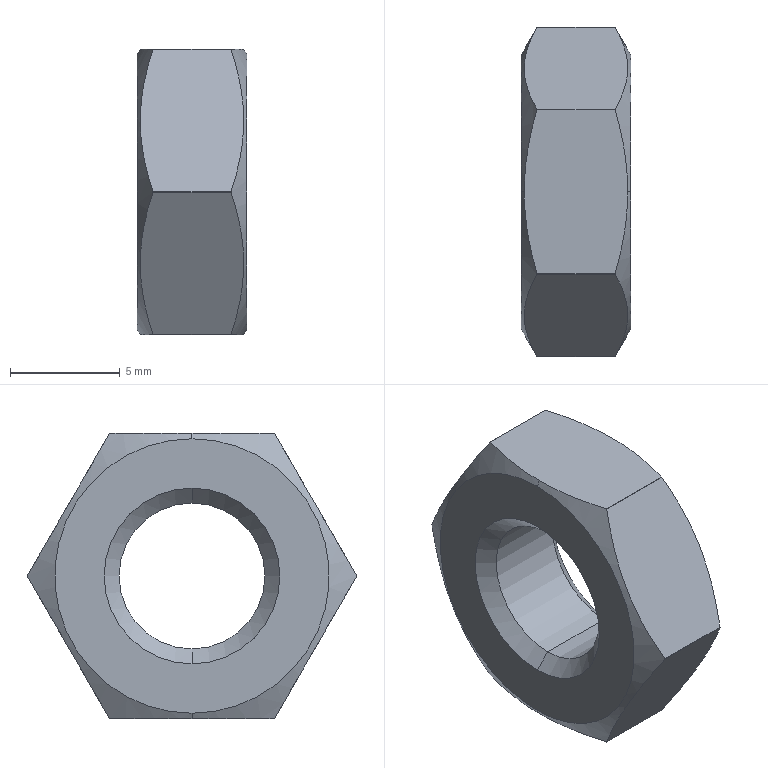Part | STEP file | Guide wheel mechanism revised.sldasm-Part-424 | 1 solid | 24 faces | box 5 x 15 x 13 mm | volume 537.919 mm3 | cone 8 | cylinder 8 | plane 8 | commonest cylinder face diameters 15 x6 6.647 x2
STEP:
#1=CARTESIAN_POINT('',(4.324,0.,-3.324));
#2=VERTEX_POINT('',#1);
#3=CARTESIAN_POINT('',(4.324,0.,3.324));
#4=VERTEX_POINT('',#3);
#5=CARTESIAN_POINT('',(4.324,0.,0.));
#6=DIRECTION('',(-1.,0.,0.));
#7=DIRECTION('',(0.,0.,1.));
#8=AXIS2_PLACEMENT_3D('',#5,#6,#7);
#9=CIRCLE('',#8,3.324);
#10=EDGE_CURVE('',#2,#4,#9,.T.);
#11=ORIENTED_EDGE('',*,*,#10,.T.);
#12=CARTESIAN_POINT('',(5.,0.,4.));
#13=VERTEX_POINT('',#12);
#14=CARTESIAN_POINT('',(5.,0.,4.));
#15=DIRECTION('',(0.7071,0.,0.7071));
#16=VECTOR('',#15,1000.);
#17=LINE('',#14,#16);
#18=EDGE_CURVE('',#4,#13,#17,.T.);
#19=ORIENTED_EDGE('',*,*,#18,.T.);
#20=CARTESIAN_POINT('',(5.,0.,-4.));
#21=VERTEX_POINT('',#20);
#22=CARTESIAN_POINT('',(5.,0.,0.));
#23=DIRECTION('',(-1.,0.,0.));
#24=DIRECTION('',(0.,0.,1.));
#25=AXIS2_PLACEMENT_3D('',#22,#23,#24);
#26=CIRCLE('',#25,4.);
#27=EDGE_CURVE('',#21,#13,#26,.T.);
#28=ORIENTED_EDGE('',*,*,#27,.F.);
#29=CARTESIAN_POINT('',(5.,0.,-4.));
#30=DIRECTION('',(0.7071,0.,-0.7071));
#31=VECTOR('',#30,1000.);
#32=LINE('',#29,#31);
#33=EDGE_CURVE('',#2,#21,#32,.T.);
#34=ORIENTED_EDGE('',*,*,#33,.F.);
#35=EDGE_LOOP('',(#11,#19,#28,#34));
#36=FACE_OUTER_BOUND('',#35,.T.);
#37=CARTESIAN_POINT('',(5.,0.,0.));
#38=DIRECTION('',(1.,0.,0.));
#39=DIRECTION('',(0.,0.,-1.));
#40=AXIS2_PLACEMENT_3D('',#37,#38,#39);
#41=CONICAL_SURFACE('',#40,4.,0.7854);
#42=ADVANCED_FACE('',(#36),#41,.F.);
#43=ORIENTED_EDGE('',*,*,#10,.F.);
#44=CARTESIAN_POINT('',(0.6765,0.,-3.324));
#45=VERTEX_POINT('',#44);
#46=CARTESIAN_POINT('',(5.,0.,-3.324));
#47=DIRECTION('',(-1.,0.,0.));
#48=VECTOR('',#47,1000.);
#49=LINE('',#46,#48);
#50=EDGE_CURVE('',#2,#45,#49,.T.);
#51=ORIENTED_EDGE('',*,*,#50,.T.);
#52=CARTESIAN_POINT('',(0.6765,0.,3.324));
#53=VERTEX_POINT('',#52);
#54=CARTESIAN_POINT('',(0.6765,0.,0.));
#55=DIRECTION('',(-1.,0.,0.));
#56=DIRECTION('',(0.,0.,1.));
#57=AXIS2_PLACEMENT_3D('',#54,#55,#56);
#58=CIRCLE('',#57,3.324);
#59=EDGE_CURVE('',#45,#53,#58,.T.);
#60=ORIENTED_EDGE('',*,*,#59,.T.);
#61=CARTESIAN_POINT('',(5.,0.,3.324));
#62=DIRECTION('',(-1.,0.,0.));
#63=VECTOR('',#62,1000.);
#64=LINE('',#61,#63);
#65=EDGE_CURVE('',#4,#53,#64,.T.);
#66=ORIENTED_EDGE('',*,*,#65,.F.);
#67=EDGE_LOOP('',(#43,#51,#60,#66));
#68=FACE_OUTER_BOUND('',#67,.T.);
#69=CARTESIAN_POINT('',(5.,0.,0.));
#70=DIRECTION('',(-1.,0.,0.));
#71=DIRECTION('',(0.,0.,1.));
#72=AXIS2_PLACEMENT_3D('',#69,#70,#71);
#73=CYLINDRICAL_SURFACE('',#72,3.324);
#74=ADVANCED_FACE('',(#68),#73,.F.);
#75=ORIENTED_EDGE('',*,*,#59,.F.);
#76=CARTESIAN_POINT('',(0.,0.,-4.));
#77=VERTEX_POINT('',#76);
#78=CARTESIAN_POINT('',(0.6765,0.,-3.324));
#79=DIRECTION('',(-0.7071,0.,-0.7071));
#80=VECTOR('',#79,1000.);
#81=LINE('',#78,#80);
#82=EDGE_CURVE('',#45,#77,#81,.T.);
#83=ORIENTED_EDGE('',*,*,#82,.T.);
#84=CARTESIAN_POINT('',(0.,0.,4.));
#85=VERTEX_POINT('',#84);
#86=CARTESIAN_POINT('',(0.,0.,0.));
#87=DIRECTION('',(-1.,0.,0.));
#88=DIRECTION('',(0.,0.,1.));
#89=AXIS2_PLACEMENT_3D('',#86,#87,#88);
#90=CIRCLE('',#89,4.);
#91=EDGE_CURVE('',#77,#85,#90,.T.);
#92=ORIENTED_EDGE('',*,*,#91,.T.);
#93=CARTESIAN_POINT('',(0.6765,0.,3.324));
#94=DIRECTION('',(-0.7071,0.,0.7071));
#95=VECTOR('',#94,1000.);
#96=LINE('',#93,#95);
#97=EDGE_CURVE('',#53,#85,#96,.T.);
#98=ORIENTED_EDGE('',*,*,#97,.F.);
#99=EDGE_LOOP('',(#75,#83,#92,#98));
#100=FACE_OUTER_BOUND('',#99,.T.);
#101=CARTESIAN_POINT('',(0.6765,0.,0.));
#102=DIRECTION('',(-1.,0.,0.));
#103=DIRECTION('',(0.,0.,1.));
#104=AXIS2_PLACEMENT_3D('',#101,#102,#103);
#105=CONICAL_SURFACE('',#104,3.324,0.7854);
#106=ADVANCED_FACE('',(#100),#105,.F.);
#107=CARTESIAN_POINT('',(5.,0.,6.25));
#108=VERTEX_POINT('',#107);
#109=CARTESIAN_POINT('',(5.,0.,-6.25));
#110=VERTEX_POINT('',#109);
#111=CARTESIAN_POINT('',(5.,0.,0.));
#112=DIRECTION('',(-1.,0.,0.));
#113=DIRECTION('',(0.,0.,1.));
#114=AXIS2_PLACEMENT_3D('',#111,#112,#113);
#115=CIRCLE('',#114,6.25);
#116=EDGE_CURVE('',#108,#110,#115,.T.);
#117=ORIENTED_EDGE('',*,*,#116,.T.);
#118=CARTESIAN_POINT('',(4.856,0.,-6.5));
#119=VERTEX_POINT('',#118);
#120=CARTESIAN_POINT('',(5.,0.,-6.25));
#121=DIRECTION('',(-0.5,0.,-0.866));
#122=VECTOR('',#121,1000.);
#123=LINE('',#120,#122);
#124=EDGE_CURVE('',#110,#119,#123,.T.);
#125=ORIENTED_EDGE('',*,*,#124,.T.);
#126=CARTESIAN_POINT('',(4.278,3.742,-6.5));
#127=VERTEX_POINT('',#126);
#128=CARTESIAN_POINT('',(4.856,0.,-6.5));
#129=CARTESIAN_POINT('',(4.856,0.6325,-6.5));
#130=CARTESIAN_POINT('',(4.8,1.274,-6.5));
#131=CARTESIAN_POINT('',(4.598,2.524,-6.5));
#132=CARTESIAN_POINT('',(4.453,3.137,-6.5));
#133=CARTESIAN_POINT('',(4.278,3.742,-6.5));
#134=B_SPLINE_CURVE_WITH_KNOTS('',3,(#128,#129,#130,#131,#132,#133),.UNSPECIFIED.,.F.,.F.,(4,2,4),(0.01047,0.01236,0.01426),.UNSPECIFIED.);
#135=EDGE_CURVE('',#119,#127,#134,.T.);
#136=ORIENTED_EDGE('',*,*,#135,.T.);
#137=CARTESIAN_POINT('',(4.278,3.758,-6.49));
#138=VERTEX_POINT('',#137);
#139=CARTESIAN_POINT('',(4.278,0.,0.));
#140=DIRECTION('',(-1.,0.,0.));
#141=DIRECTION('',(0.,0.,1.));
#142=AXIS2_PLACEMENT_3D('',#139,#140,#141);
#143=CIRCLE('',#142,7.5);
#144=EDGE_CURVE('',#138,#127,#143,.T.);
#145=ORIENTED_EDGE('',*,*,#144,.F.);
#146=CARTESIAN_POINT('',(4.278,7.5,-0.00963));
#147=VERTEX_POINT('',#146);
#148=CARTESIAN_POINT('',(4.278,3.758,-6.49));
#149=CARTESIAN_POINT('',(4.454,4.064,-5.961));
#150=CARTESIAN_POINT('',(4.599,4.372,-5.428));
#151=CARTESIAN_POINT('',(4.8,4.993,-4.351));
#152=CARTESIAN_POINT('',(4.855,5.307,-3.807));
#153=CARTESIAN_POINT('',(4.856,5.785,-2.981));
#154=CARTESIAN_POINT('',(4.842,5.944,-2.704));
#155=CARTESIAN_POINT('',(4.79,6.26,-2.157));
#156=CARTESIAN_POINT('',(4.751,6.417,-1.885));
#157=CARTESIAN_POINT('',(4.6,6.886,-1.074));
#158=CARTESIAN_POINT('',(4.455,7.194,-0.5394));
#159=CARTESIAN_POINT('',(4.278,7.5,-0.00963));
#160=B_SPLINE_CURVE_WITH_KNOTS('',3,(#148,#149,#150,#151,#152,#153,#154,#155,#156,#157,#158,#159),.UNSPECIFIED.,.F.,.F.,(4,2,2,2,2,4),(0.000000716,0.00189,0.003779,0.004724,0.005668,0.007558),.UNSPECIFIED.);
#161=EDGE_CURVE('',#138,#147,#160,.T.);
#162=ORIENTED_EDGE('',*,*,#161,.T.);
#163=CARTESIAN_POINT('',(4.278,7.5,0.00963));
#164=VERTEX_POINT('',#163);
#165=CARTESIAN_POINT('',(4.278,0.,0.));
#166=DIRECTION('',(-1.,0.,0.));
#167=DIRECTION('',(0.,0.,1.));
#168=AXIS2_PLACEMENT_3D('',#165,#166,#167);
#169=CIRCLE('',#168,7.5);
#170=EDGE_CURVE('',#164,#147,#169,.T.);
#171=ORIENTED_EDGE('',*,*,#170,.F.);
#172=CARTESIAN_POINT('',(4.278,3.758,6.49));
#173=VERTEX_POINT('',#172);
#174=CARTESIAN_POINT('',(4.278,7.5,0.00963));
#175=CARTESIAN_POINT('',(4.454,7.194,0.5388));
#176=CARTESIAN_POINT('',(4.599,6.887,1.072));
#177=CARTESIAN_POINT('',(4.8,6.265,2.149));
#178=CARTESIAN_POINT('',(4.855,5.951,2.693));
#179=CARTESIAN_POINT('',(4.856,5.474,3.519));
#180=CARTESIAN_POINT('',(4.842,5.314,3.796));
#181=CARTESIAN_POINT('',(4.79,4.998,4.343));
#182=CARTESIAN_POINT('',(4.751,4.841,4.615));
#183=CARTESIAN_POINT('',(4.6,4.373,5.426));
#184=CARTESIAN_POINT('',(4.455,4.064,5.961));
#185=CARTESIAN_POINT('',(4.278,3.758,6.49));
#186=B_SPLINE_CURVE_WITH_KNOTS('',3,(#174,#175,#176,#177,#178,#179,#180,#181,#182,#183,#184,#185),.UNSPECIFIED.,.F.,.F.,(4,2,2,2,2,4),(0.000000425,0.00189,0.003779,0.004723,0.005668,0.007557),.UNSPECIFIED.);
#187=EDGE_CURVE('',#164,#173,#186,.T.);
#188=ORIENTED_EDGE('',*,*,#187,.T.);
#189=CARTESIAN_POINT('',(4.278,3.742,6.5));
#190=VERTEX_POINT('',#189);
#191=CARTESIAN_POINT('',(4.278,0.,0.));
#192=DIRECTION('',(-1.,0.,0.));
#193=DIRECTION('',(0.,0.,1.));
#194=AXIS2_PLACEMENT_3D('',#191,#192,#193);
#195=CIRCLE('',#194,7.5);
#196=EDGE_CURVE('',#190,#173,#195,.T.);
#197=ORIENTED_EDGE('',*,*,#196,.F.);
#198=CARTESIAN_POINT('',(4.856,0.,6.5));
#199=VERTEX_POINT('',#198);
#200=CARTESIAN_POINT('',(4.278,3.742,6.5));
#201=CARTESIAN_POINT('',(4.453,3.137,6.5));
#202=CARTESIAN_POINT('',(4.598,2.524,6.5));
#203=CARTESIAN_POINT('',(4.8,1.274,6.5));
#204=CARTESIAN_POINT('',(4.856,0.6325,6.5));
#205=CARTESIAN_POINT('',(4.856,0.,6.5));
#206=B_SPLINE_CURVE_WITH_KNOTS('',3,(#200,#201,#202,#203,#204,#205),.UNSPECIFIED.,.F.,.F.,(4,2,4),(0.002787,0.004676,0.006564),.UNSPECIFIED.);
#207=EDGE_CURVE('',#190,#199,#206,.T.);
#208=ORIENTED_EDGE('',*,*,#207,.T.);
#209=CARTESIAN_POINT('',(5.,0.,6.25));
#210=DIRECTION('',(-0.5,0.,0.866));
#211=VECTOR('',#210,1000.);
#212=LINE('',#209,#211);
#213=EDGE_CURVE('',#108,#199,#212,.T.);
#214=ORIENTED_EDGE('',*,*,#213,.F.);
#215=EDGE_LOOP('',(#117,#125,#136,#145,#162,#171,#188,#197,#208,#214));
#216=FACE_OUTER_BOUND('',#215,.T.);
#217=CARTESIAN_POINT('',(5.,0.,0.));
#218=DIRECTION('',(-1.,0.,0.));
#219=DIRECTION('',(0.,0.,1.));
#220=AXIS2_PLACEMENT_3D('',#217,#218,#219);
#221=CONICAL_SURFACE('',#220,6.25,1.047);
#222=ADVANCED_FACE('',(#216),#221,.T.);
#223=CARTESIAN_POINT('',(0.,0.,6.25));
#224=VERTEX_POINT('',#223);
#225=CARTESIAN_POINT('',(0.,0.,-6.25));
#226=VERTEX_POINT('',#225);
#227=CARTESIAN_POINT('',(0.,0.,0.));
#228=DIRECTION('',(-1.,0.,0.));
#229=DIRECTION('',(0.,0.,1.));
#230=AXIS2_PLACEMENT_3D('',#227,#228,#229);
#231=CIRCLE('',#230,6.25);
#232=EDGE_CURVE('',#224,#226,#231,.T.);
#233=ORIENTED_EDGE('',*,*,#232,.F.);
#234=CARTESIAN_POINT('',(0.1443,0.,6.5));
#235=VERTEX_POINT('',#234);
#236=CARTESIAN_POINT('',(0.7217,0.,7.5));
#237=DIRECTION('',(0.5,0.,0.866));
#238=VECTOR('',#237,1000.);
#239=LINE('',#236,#238);
#240=EDGE_CURVE('',#224,#235,#239,.T.);
#241=ORIENTED_EDGE('',*,*,#240,.T.);
#242=CARTESIAN_POINT('',(0.7217,3.742,6.5));
#243=VERTEX_POINT('',#242);
#244=CARTESIAN_POINT('',(0.1443,0.,6.5));
#245=CARTESIAN_POINT('',(0.1443,0.6325,6.5));
#246=CARTESIAN_POINT('',(0.2,1.274,6.5));
#247=CARTESIAN_POINT('',(0.4023,2.524,6.5));
#248=CARTESIAN_POINT('',(0.5474,3.137,6.5));
#249=CARTESIAN_POINT('',(0.7217,3.742,6.5));
#250=B_SPLINE_CURVE_WITH_KNOTS('',3,(#244,#245,#246,#247,#248,#249),.UNSPECIFIED.,.F.,.F.,(4,2,4),(0.01047,0.01236,0.01426),.UNSPECIFIED.);
#251=EDGE_CURVE('',#235,#243,#250,.T.);
#252=ORIENTED_EDGE('',*,*,#251,.T.);
#253=CARTESIAN_POINT('',(0.7217,3.758,6.49));
#254=VERTEX_POINT('',#253);
#255=CARTESIAN_POINT('',(0.7217,0.,0.));
#256=DIRECTION('',(-1.,0.,0.));
#257=DIRECTION('',(0.,0.,1.));
#258=AXIS2_PLACEMENT_3D('',#255,#256,#257);
#259=CIRCLE('',#258,7.5);
#260=EDGE_CURVE('',#243,#254,#259,.T.);
#261=ORIENTED_EDGE('',*,*,#260,.T.);
#262=CARTESIAN_POINT('',(0.7217,7.5,0.00963));
#263=VERTEX_POINT('',#262);
#264=CARTESIAN_POINT('',(0.7217,3.758,6.49));
#265=CARTESIAN_POINT('',(0.5457,4.064,5.961));
#266=CARTESIAN_POINT('',(0.4007,4.372,5.428));
#267=CARTESIAN_POINT('',(0.1999,4.993,4.351));
#268=CARTESIAN_POINT('',(0.1448,5.307,3.807));
#269=CARTESIAN_POINT('',(0.1441,5.785,2.981));
#270=CARTESIAN_POINT('',(0.1576,5.944,2.704));
#271=CARTESIAN_POINT('',(0.2102,6.26,2.157));
#272=CARTESIAN_POINT('',(0.2493,6.417,1.885));
#273=CARTESIAN_POINT('',(0.4001,6.886,1.074));
#274=CARTESIAN_POINT('',(0.5455,7.194,0.5394));
#275=CARTESIAN_POINT('',(0.7217,7.5,0.00963));
#276=B_SPLINE_CURVE_WITH_KNOTS('',3,(#264,#265,#266,#267,#268,#269,#270,#271,#272,#273,#274,#275),.UNSPECIFIED.,.F.,.F.,(4,2,2,2,2,4),(0.000000716,0.00189,0.003779,0.004724,0.005668,0.007558),.UNSPECIFIED.);
#277=EDGE_CURVE('',#254,#263,#276,.T.);
#278=ORIENTED_EDGE('',*,*,#277,.T.);
#279=CARTESIAN_POINT('',(0.7217,7.5,-0.00963));
#280=VERTEX_POINT('',#279);
#281=CARTESIAN_POINT('',(0.7217,0.,0.));
#282=DIRECTION('',(-1.,0.,0.));
#283=DIRECTION('',(0.,0.,1.));
#284=AXIS2_PLACEMENT_3D('',#281,#282,#283);
#285=CIRCLE('',#284,7.5);
#286=EDGE_CURVE('',#263,#280,#285,.T.);
#287=ORIENTED_EDGE('',*,*,#286,.T.);
#288=CARTESIAN_POINT('',(0.7217,3.758,-6.49));
#289=VERTEX_POINT('',#288);
#290=CARTESIAN_POINT('',(0.7217,7.5,-0.00963));
#291=CARTESIAN_POINT('',(0.5457,7.194,-0.5388));
#292=CARTESIAN_POINT('',(0.4007,6.887,-1.072));
#293=CARTESIAN_POINT('',(0.1999,6.265,-2.149));
#294=CARTESIAN_POINT('',(0.1448,5.951,-2.693));
#295=CARTESIAN_POINT('',(0.1441,5.474,-3.519));
#296=CARTESIAN_POINT('',(0.1576,5.314,-3.796));
#297=CARTESIAN_POINT('',(0.2102,4.998,-4.343));
#298=CARTESIAN_POINT('',(0.2493,4.841,-4.615));
#299=CARTESIAN_POINT('',(0.4001,4.373,-5.426));
#300=CARTESIAN_POINT('',(0.5455,4.064,-5.961));
#301=CARTESIAN_POINT('',(0.7217,3.758,-6.49));
#302=B_SPLINE_CURVE_WITH_KNOTS('',3,(#290,#291,#292,#293,#294,#295,#296,#297,#298,#299,#300,#301),.UNSPECIFIED.,.F.,.F.,(4,2,2,2,2,4),(0.000000425,0.00189,0.003779,0.004723,0.005668,0.007557),.UNSPECIFIED.);
#303=EDGE_CURVE('',#280,#289,#302,.T.);
#304=ORIENTED_EDGE('',*,*,#303,.T.);
#305=CARTESIAN_POINT('',(0.7217,3.742,-6.5));
#306=VERTEX_POINT('',#305);
#307=CARTESIAN_POINT('',(0.7217,0.,0.));
#308=DIRECTION('',(-1.,0.,0.));
#309=DIRECTION('',(0.,0.,1.));
#310=AXIS2_PLACEMENT_3D('',#307,#308,#309);
#311=CIRCLE('',#310,7.5);
#312=EDGE_CURVE('',#289,#306,#311,.T.);
#313=ORIENTED_EDGE('',*,*,#312,.T.);
#314=CARTESIAN_POINT('',(0.1443,0.,-6.5));
#315=VERTEX_POINT('',#314);
#316=CARTESIAN_POINT('',(0.7217,3.742,-6.5));
#317=CARTESIAN_POINT('',(0.5474,3.137,-6.5));
#318=CARTESIAN_POINT('',(0.4023,2.524,-6.5));
#319=CARTESIAN_POINT('',(0.2,1.274,-6.5));
#320=CARTESIAN_POINT('',(0.1443,0.6325,-6.5));
#321=CARTESIAN_POINT('',(0.1443,0.,-6.5));
#322=B_SPLINE_CURVE_WITH_KNOTS('',3,(#316,#317,#318,#319,#320,#321),.UNSPECIFIED.,.F.,.F.,(4,2,4),(0.002787,0.004676,0.006564),.UNSPECIFIED.);
#323=EDGE_CURVE('',#306,#315,#322,.T.);
#324=ORIENTED_EDGE('',*,*,#323,.T.);
#325=CARTESIAN_POINT('',(0.7217,0.,-7.5));
#326=DIRECTION('',(0.5,0.,-0.866));
#327=VECTOR('',#326,1000.);
#328=LINE('',#325,#327);
#329=EDGE_CURVE('',#226,#315,#328,.T.);
#330=ORIENTED_EDGE('',*,*,#329,.F.);
#331=EDGE_LOOP('',(#233,#241,#252,#261,#278,#287,#304,#313,#324,#330));
#332=FACE_OUTER_BOUND('',#331,.T.);
#333=CARTESIAN_POINT('',(0.7217,0.,0.));
#334=DIRECTION('',(1.,0.,0.));
#335=DIRECTION('',(0.,0.,-1.));
#336=AXIS2_PLACEMENT_3D('',#333,#334,#335);
#337=CONICAL_SURFACE('',#336,7.5,1.047);
#338=ADVANCED_FACE('',(#332),#337,.T.);
#339=CARTESIAN_POINT('',(0.,0.,0.));
#340=DIRECTION('',(-1.,0.,0.));
#341=DIRECTION('',(0.,0.,1.));
#342=AXIS2_PLACEMENT_3D('',#339,#340,#341);
#343=CIRCLE('',#342,6.25);
#344=EDGE_CURVE('',#226,#224,#343,.T.);
#345=ORIENTED_EDGE('',*,*,#344,.T.);
#346=ORIENTED_EDGE('',*,*,#232,.T.);
#347=EDGE_LOOP('',(#345,#346));
#348=FACE_OUTER_BOUND('',#347,.T.);
#349=CARTESIAN_POINT('',(0.,0.,0.));
#350=DIRECTION('',(-1.,0.,0.));
#351=DIRECTION('',(0.,0.,1.));
#352=AXIS2_PLACEMENT_3D('',#349,#350,#351);
#353=CIRCLE('',#352,4.);
#354=EDGE_CURVE('',#85,#77,#353,.T.);
#355=ORIENTED_EDGE('',*,*,#354,.F.);
#356=ORIENTED_EDGE('',*,*,#91,.F.);
#357=EDGE_LOOP('',(#355,#356));
#358=FACE_BOUND('',#357,.T.);
#359=CARTESIAN_POINT('',(0.,0.,0.));
#360=DIRECTION('',(1.,0.,0.));
#361=DIRECTION('',(0.,0.,-1.));
#362=AXIS2_PLACEMENT_3D('',#359,#360,#361);
#363=PLANE('',#362);
#364=ADVANCED_FACE('',(#348,#358),#363,.F.);
#365=ORIENTED_EDGE('',*,*,#116,.F.);
#366=CARTESIAN_POINT('',(5.,0.,0.));
#367=DIRECTION('',(-1.,0.,0.));
#368=DIRECTION('',(0.,0.,1.));
#369=AXIS2_PLACEMENT_3D('',#366,#367,#368);
#370=CIRCLE('',#369,6.25);
#371=EDGE_CURVE('',#110,#108,#370,.T.);
#372=ORIENTED_EDGE('',*,*,#371,.F.);
#373=EDGE_LOOP('',(#365,#372));
#374=FACE_OUTER_BOUND('',#373,.T.);
#375=ORIENTED_EDGE('',*,*,#27,.T.);
#376=CARTESIAN_POINT('',(5.,0.,0.));
#377=DIRECTION('',(-1.,0.,0.));
#378=DIRECTION('',(0.,0.,1.));
#379=AXIS2_PLACEMENT_3D('',#376,#377,#378);
#380=CIRCLE('',#379,4.);
#381=EDGE_CURVE('',#13,#21,#380,.T.);
#382=ORIENTED_EDGE('',*,*,#381,.T.);
#383=EDGE_LOOP('',(#375,#382));
#384=FACE_BOUND('',#383,.T.);
#385=CARTESIAN_POINT('',(5.,6.25,0.));
#386=DIRECTION('',(-1.,0.,0.));
#387=DIRECTION('',(0.,0.,1.));
#388=AXIS2_PLACEMENT_3D('',#385,#386,#387);
#389=PLANE('',#388);
#390=ADVANCED_FACE('',(#374,#384),#389,.F.);
#391=ORIENTED_EDGE('',*,*,#196,.T.);
#392=CARTESIAN_POINT('',(5.,3.758,6.49));
#393=DIRECTION('',(-1.,0.,0.));
#394=VECTOR('',#393,1000.);
#395=LINE('',#392,#394);
#396=EDGE_CURVE('',#173,#254,#395,.T.);
#397=ORIENTED_EDGE('',*,*,#396,.T.);
#398=ORIENTED_EDGE('',*,*,#260,.F.);
#399=CARTESIAN_POINT('',(5.,3.742,6.5));
#400=DIRECTION('',(1.,0.,0.));
#401=VECTOR('',#400,1000.);
#402=LINE('',#399,#401);
#403=EDGE_CURVE('',#243,#190,#402,.T.);
#404=ORIENTED_EDGE('',*,*,#403,.T.);
#405=EDGE_LOOP('',(#391,#397,#398,#404));
#406=FACE_OUTER_BOUND('',#405,.T.);
#407=CARTESIAN_POINT('',(5.,0.,0.));
#408=DIRECTION('',(-1.,0.,0.));
#409=DIRECTION('',(0.,0.,1.));
#410=AXIS2_PLACEMENT_3D('',#407,#408,#409);
#411=CYLINDRICAL_SURFACE('',#410,7.5);
#412=ADVANCED_FACE('',(#406),#411,.T.);
#413=CARTESIAN_POINT('',(4.278,-3.758,6.49));
#414=VERTEX_POINT('',#413);
#415=CARTESIAN_POINT('',(4.278,-3.742,6.5));
#416=VERTEX_POINT('',#415);
#417=CARTESIAN_POINT('',(4.278,0.,0.));
#418=DIRECTION('',(-1.,0.,0.));
#419=DIRECTION('',(0.,0.,1.));
#420=AXIS2_PLACEMENT_3D('',#417,#418,#419);
#421=CIRCLE('',#420,7.5);
#422=EDGE_CURVE('',#414,#416,#421,.T.);
#423=ORIENTED_EDGE('',*,*,#422,.T.);
#424=CARTESIAN_POINT('',(0.7217,-3.742,6.5));
#425=VERTEX_POINT('',#424);
#426=CARTESIAN_POINT('',(5.,-3.742,6.5));
#427=DIRECTION('',(-1.,0.,0.));
#428=VECTOR('',#427,1000.);
#429=LINE('',#426,#428);
#430=EDGE_CURVE('',#416,#425,#429,.T.);
#431=ORIENTED_EDGE('',*,*,#430,.T.);
#432=CARTESIAN_POINT('',(0.7217,-3.758,6.49));
#433=VERTEX_POINT('',#432);
#434=CARTESIAN_POINT('',(0.7217,0.,0.));
#435=DIRECTION('',(-1.,0.,0.));
#436=DIRECTION('',(0.,0.,1.));
#437=AXIS2_PLACEMENT_3D('',#434,#435,#436);
#438=CIRCLE('',#437,7.5);
#439=EDGE_CURVE('',#433,#425,#438,.T.);
#440=ORIENTED_EDGE('',*,*,#439,.F.);
#441=CARTESIAN_POINT('',(5.,-3.758,6.49));
#442=DIRECTION('',(1.,0.,0.));
#443=VECTOR('',#442,1000.);
#444=LINE('',#441,#443);
#445=EDGE_CURVE('',#433,#414,#444,.T.);
#446=ORIENTED_EDGE('',*,*,#445,.T.);
#447=EDGE_LOOP('',(#423,#431,#440,#446));
#448=FACE_OUTER_BOUND('',#447,.T.);
#449=CARTESIAN_POINT('',(5.,0.,0.));
#450=DIRECTION('',(-1.,0.,0.));
#451=DIRECTION('',(0.,0.,1.));
#452=AXIS2_PLACEMENT_3D('',#449,#450,#451);
#453=CYLINDRICAL_SURFACE('',#452,7.5);
#454=ADVANCED_FACE('',(#448),#453,.T.);
#455=CARTESIAN_POINT('',(4.278,-7.5,-0.00963));
#456=VERTEX_POINT('',#455);
#457=CARTESIAN_POINT('',(4.278,-7.5,0.00963));
#458=VERTEX_POINT('',#457);
#459=CARTESIAN_POINT('',(4.278,0.,0.));
#460=DIRECTION('',(-1.,0.,0.));
#461=DIRECTION('',(0.,0.,1.));
#462=AXIS2_PLACEMENT_3D('',#459,#460,#461);
#463=CIRCLE('',#462,7.5);
#464=EDGE_CURVE('',#456,#458,#463,.T.);
#465=ORIENTED_EDGE('',*,*,#464,.T.);
#466=CARTESIAN_POINT('',(0.7217,-7.5,0.00963));
#467=VERTEX_POINT('',#466);
#468=CARTESIAN_POINT('',(5.,-7.5,0.00963));
#469=DIRECTION('',(-1.,0.,0.));
#470=VECTOR('',#469,1000.);
#471=LINE('',#468,#470);
#472=EDGE_CURVE('',#458,#467,#471,.T.);
#473=ORIENTED_EDGE('',*,*,#472,.T.);
#474=CARTESIAN_POINT('',(0.7217,-7.5,-0.00963));
#475=VERTEX_POINT('',#474);
#476=CARTESIAN_POINT('',(0.7217,0.,0.));
#477=DIRECTION('',(-1.,0.,0.));
#478=DIRECTION('',(0.,0.,1.));
#479=AXIS2_PLACEMENT_3D('',#476,#477,#478);
#480=CIRCLE('',#479,7.5);
#481=EDGE_CURVE('',#475,#467,#480,.T.);
#482=ORIENTED_EDGE('',*,*,#481,.F.);
#483=CARTESIAN_POINT('',(5.,-7.5,-0.00963));
#484=DIRECTION('',(1.,0.,0.));
#485=VECTOR('',#484,1000.);
#486=LINE('',#483,#485);
#487=EDGE_CURVE('',#475,#456,#486,.T.);
#488=ORIENTED_EDGE('',*,*,#487,.T.);
#489=EDGE_LOOP('',(#465,#473,#482,#488));
#490=FACE_OUTER_BOUND('',#489,.T.);
#491=CARTESIAN_POINT('',(5.,0.,0.));
#492=DIRECTION('',(-1.,0.,0.));
#493=DIRECTION('',(0.,0.,1.));
#494=AXIS2_PLACEMENT_3D('',#491,#492,#493);
#495=CYLINDRICAL_SURFACE('',#494,7.5);
#496=ADVANCED_FACE('',(#490),#495,.T.);
#497=CARTESIAN_POINT('',(4.278,-3.742,-6.5));
#498=VERTEX_POINT('',#497);
#499=CARTESIAN_POINT('',(4.278,-3.758,-6.49));
#500=VERTEX_POINT('',#499);
#501=CARTESIAN_POINT('',(4.278,0.,0.));
#502=DIRECTION('',(-1.,0.,0.));
#503=DIRECTION('',(0.,0.,1.));
#504=AXIS2_PLACEMENT_3D('',#501,#502,#503);
#505=CIRCLE('',#504,7.5);
#506=EDGE_CURVE('',#498,#500,#505,.T.);
#507=ORIENTED_EDGE('',*,*,#506,.T.);
#508=CARTESIAN_POINT('',(0.7217,-3.758,-6.49));
#509=VERTEX_POINT('',#508);
#510=CARTESIAN_POINT('',(5.,-3.758,-6.49));
#511=DIRECTION('',(-1.,0.,0.));
#512=VECTOR('',#511,1000.);
#513=LINE('',#510,#512);
#514=EDGE_CURVE('',#500,#509,#513,.T.);
#515=ORIENTED_EDGE('',*,*,#514,.T.);
#516=CARTESIAN_POINT('',(0.7217,-3.742,-6.5));
#517=VERTEX_POINT('',#516);
#518=CARTESIAN_POINT('',(0.7217,0.,0.));
#519=DIRECTION('',(-1.,0.,0.));
#520=DIRECTION('',(0.,0.,1.));
#521=AXIS2_PLACEMENT_3D('',#518,#519,#520);
#522=CIRCLE('',#521,7.5);
#523=EDGE_CURVE('',#517,#509,#522,.T.);
#524=ORIENTED_EDGE('',*,*,#523,.F.);
#525=CARTESIAN_POINT('',(5.,-3.742,-6.5));
#526=DIRECTION('',(1.,0.,0.));
#527=VECTOR('',#526,1000.);
#528=LINE('',#525,#527);
#529=EDGE_CURVE('',#517,#498,#528,.T.);
#530=ORIENTED_EDGE('',*,*,#529,.T.);
#531=EDGE_LOOP('',(#507,#515,#524,#530));
#532=FACE_OUTER_BOUND('',#531,.T.);
#533=CARTESIAN_POINT('',(5.,0.,0.));
#534=DIRECTION('',(-1.,0.,0.));
#535=DIRECTION('',(0.,0.,1.));
#536=AXIS2_PLACEMENT_3D('',#533,#534,#535);
#537=CYLINDRICAL_SURFACE('',#536,7.5);
#538=ADVANCED_FACE('',(#532),#537,.T.);
#539=ORIENTED_EDGE('',*,*,#144,.T.);
#540=CARTESIAN_POINT('',(5.,3.742,-6.5));
#541=DIRECTION('',(-1.,0.,0.));
#542=VECTOR('',#541,1000.);
#543=LINE('',#540,#542);
#544=EDGE_CURVE('',#127,#306,#543,.T.);
#545=ORIENTED_EDGE('',*,*,#544,.T.);
#546=ORIENTED_EDGE('',*,*,#312,.F.);
#547=CARTESIAN_POINT('',(5.,3.758,-6.49));
#548=DIRECTION('',(1.,0.,0.));
#549=VECTOR('',#548,1000.);
#550=LINE('',#547,#549);
#551=EDGE_CURVE('',#289,#138,#550,.T.);
#552=ORIENTED_EDGE('',*,*,#551,.T.);
#553=EDGE_LOOP('',(#539,#545,#546,#552));
#554=FACE_OUTER_BOUND('',#553,.T.);
#555=CARTESIAN_POINT('',(5.,0.,0.));
#556=DIRECTION('',(-1.,0.,0.));
#557=DIRECTION('',(0.,0.,1.));
#558=AXIS2_PLACEMENT_3D('',#555,#556,#557);
#559=CYLINDRICAL_SURFACE('',#558,7.5);
#560=ADVANCED_FACE('',(#554),#559,.T.);
#561=ORIENTED_EDGE('',*,*,#240,.F.);
#562=ORIENTED_EDGE('',*,*,#344,.F.);
#563=ORIENTED_EDGE('',*,*,#329,.T.);
#564=CARTESIAN_POINT('',(0.1443,0.,-6.5));
#565=CARTESIAN_POINT('',(0.1443,-0.6322,-6.5));
#566=CARTESIAN_POINT('',(0.1985,-1.26,-6.5));
#567=CARTESIAN_POINT('',(0.3994,-2.51,-6.5));
#568=CARTESIAN_POINT('',(0.5464,-3.133,-6.5));
#569=CARTESIAN_POINT('',(0.7217,-3.742,-6.5));
#570=B_SPLINE_CURVE_WITH_KNOTS('',3,(#564,#565,#566,#567,#568,#569),.UNSPECIFIED.,.F.,.F.,(4,2,4),(0.006564,0.008452,0.01034),.UNSPECIFIED.);
#571=EDGE_CURVE('',#315,#517,#570,.T.);
#572=ORIENTED_EDGE('',*,*,#571,.T.);
#573=ORIENTED_EDGE('',*,*,#523,.T.);
#574=CARTESIAN_POINT('',(0.7217,-3.758,-6.49));
#575=CARTESIAN_POINT('',(0.5457,-4.064,-5.961));
#576=CARTESIAN_POINT('',(0.4007,-4.372,-5.428));
#577=CARTESIAN_POINT('',(0.1999,-4.993,-4.351));
#578=CARTESIAN_POINT('',(0.1448,-5.307,-3.807));
#579=CARTESIAN_POINT('',(0.1441,-5.785,-2.981));
#580=CARTESIAN_POINT('',(0.1576,-5.944,-2.704));
#581=CARTESIAN_POINT('',(0.2102,-6.26,-2.157));
#582=CARTESIAN_POINT('',(0.2493,-6.417,-1.885));
#583=CARTESIAN_POINT('',(0.4001,-6.886,-1.074));
#584=CARTESIAN_POINT('',(0.5455,-7.194,-0.5394));
#585=CARTESIAN_POINT('',(0.7217,-7.5,-0.00963));
#586=B_SPLINE_CURVE_WITH_KNOTS('',3,(#574,#575,#576,#577,#578,#579,#580,#581,#582,#583,#584,#585),.UNSPECIFIED.,.F.,.F.,(4,2,2,2,2,4),(0.000000716,0.00189,0.003779,0.004724,0.005668,0.007558),.UNSPECIFIED.);
#587=EDGE_CURVE('',#509,#475,#586,.T.);
#588=ORIENTED_EDGE('',*,*,#587,.T.);
#589=ORIENTED_EDGE('',*,*,#481,.T.);
#590=CARTESIAN_POINT('',(0.7217,-7.5,0.00963));
#591=CARTESIAN_POINT('',(0.5457,-7.194,0.5388));
#592=CARTESIAN_POINT('',(0.4007,-6.887,1.072));
#593=CARTESIAN_POINT('',(0.1999,-6.265,2.149));
#594=CARTESIAN_POINT('',(0.1448,-5.951,2.693));
#595=CARTESIAN_POINT('',(0.1441,-5.474,3.519));
#596=CARTESIAN_POINT('',(0.1576,-5.314,3.796));
#597=CARTESIAN_POINT('',(0.2102,-4.998,4.343));
#598=CARTESIAN_POINT('',(0.2493,-4.841,4.615));
#599=CARTESIAN_POINT('',(0.4001,-4.373,5.426));
#600=CARTESIAN_POINT('',(0.5455,-4.064,5.961));
#601=CARTESIAN_POINT('',(0.7217,-3.758,6.49));
#602=B_SPLINE_CURVE_WITH_KNOTS('',3,(#590,#591,#592,#593,#594,#595,#596,#597,#598,#599,#600,#601),.UNSPECIFIED.,.F.,.F.,(4,2,2,2,2,4),(0.000000425,0.00189,0.003779,0.004723,0.005668,0.007557),.UNSPECIFIED.);
#603=EDGE_CURVE('',#467,#433,#602,.T.);
#604=ORIENTED_EDGE('',*,*,#603,.T.);
#605=ORIENTED_EDGE('',*,*,#439,.T.);
#606=CARTESIAN_POINT('',(0.7217,-3.742,6.5));
#607=CARTESIAN_POINT('',(0.5464,-3.133,6.5));
#608=CARTESIAN_POINT('',(0.3994,-2.51,6.5));
#609=CARTESIAN_POINT('',(0.1985,-1.26,6.5));
#610=CARTESIAN_POINT('',(0.1443,-0.6322,6.5));
#611=CARTESIAN_POINT('',(0.1443,0.,6.5));
#612=B_SPLINE_CURVE_WITH_KNOTS('',3,(#606,#607,#608,#609,#610,#611),.UNSPECIFIED.,.F.,.F.,(4,2,4),(0.006684,0.008577,0.01047),.UNSPECIFIED.);
#613=EDGE_CURVE('',#425,#235,#612,.T.);
#614=ORIENTED_EDGE('',*,*,#613,.T.);
#615=EDGE_LOOP('',(#561,#562,#563,#572,#573,#588,#589,#604,#605,#614));
#616=FACE_OUTER_BOUND('',#615,.T.);
#617=CARTESIAN_POINT('',(0.7217,0.,0.));
#618=DIRECTION('',(1.,0.,0.));
#619=DIRECTION('',(0.,0.,-1.));
#620=AXIS2_PLACEMENT_3D('',#617,#618,#619);
#621=CONICAL_SURFACE('',#620,7.5,1.047);
#622=ADVANCED_FACE('',(#616),#621,.T.);
#623=ORIENTED_EDGE('',*,*,#286,.F.);
#624=CARTESIAN_POINT('',(5.,7.5,0.00963));
#625=DIRECTION('',(1.,0.,0.));
#626=VECTOR('',#625,1000.);
#627=LINE('',#624,#626);
#628=EDGE_CURVE('',#263,#164,#627,.T.);
#629=ORIENTED_EDGE('',*,*,#628,.T.);
#630=ORIENTED_EDGE('',*,*,#170,.T.);
#631=CARTESIAN_POINT('',(5.,7.5,-0.00963));
#632=DIRECTION('',(-1.,0.,0.));
#633=VECTOR('',#632,1000.);
#634=LINE('',#631,#633);
#635=EDGE_CURVE('',#147,#280,#634,.T.);
#636=ORIENTED_EDGE('',*,*,#635,.T.);
#637=EDGE_LOOP('',(#623,#629,#630,#636));
#638=FACE_OUTER_BOUND('',#637,.T.);
#639=CARTESIAN_POINT('',(5.,0.,0.));
#640=DIRECTION('',(-1.,0.,0.));
#641=DIRECTION('',(0.,0.,1.));
#642=AXIS2_PLACEMENT_3D('',#639,#640,#641);
#643=CYLINDRICAL_SURFACE('',#642,7.5);
#644=ADVANCED_FACE('',(#638),#643,.T.);
#645=ORIENTED_EDGE('',*,*,#124,.F.);
#646=ORIENTED_EDGE('',*,*,#371,.T.);
#647=ORIENTED_EDGE('',*,*,#213,.T.);
#648=CARTESIAN_POINT('',(4.856,0.,6.5));
#649=CARTESIAN_POINT('',(4.856,-0.6322,6.5));
#650=CARTESIAN_POINT('',(4.801,-1.26,6.5));
#651=CARTESIAN_POINT('',(4.601,-2.51,6.5));
#652=CARTESIAN_POINT('',(4.454,-3.133,6.5));
#653=CARTESIAN_POINT('',(4.278,-3.742,6.5));
#654=B_SPLINE_CURVE_WITH_KNOTS('',3,(#648,#649,#650,#651,#652,#653),.UNSPECIFIED.,.F.,.F.,(4,2,4),(0.006564,0.008452,0.01034),.UNSPECIFIED.);
#655=EDGE_CURVE('',#199,#416,#654,.T.);
#656=ORIENTED_EDGE('',*,*,#655,.T.);
#657=ORIENTED_EDGE('',*,*,#422,.F.);
#658=CARTESIAN_POINT('',(4.278,-3.758,6.49));
#659=CARTESIAN_POINT('',(4.454,-4.064,5.961));
#660=CARTESIAN_POINT('',(4.599,-4.372,5.428));
#661=CARTESIAN_POINT('',(4.8,-4.993,4.351));
#662=CARTESIAN_POINT('',(4.855,-5.307,3.807));
#663=CARTESIAN_POINT('',(4.856,-5.785,2.981));
#664=CARTESIAN_POINT('',(4.842,-5.944,2.704));
#665=CARTESIAN_POINT('',(4.79,-6.26,2.157));
#666=CARTESIAN_POINT('',(4.751,-6.417,1.885));
#667=CARTESIAN_POINT('',(4.6,-6.886,1.074));
#668=CARTESIAN_POINT('',(4.455,-7.194,0.5394));
#669=CARTESIAN_POINT('',(4.278,-7.5,0.00963));
#670=B_SPLINE_CURVE_WITH_KNOTS('',3,(#658,#659,#660,#661,#662,#663,#664,#665,#666,#667,#668,#669),.UNSPECIFIED.,.F.,.F.,(4,2,2,2,2,4),(0.000000716,0.00189,0.003779,0.004724,0.005668,0.007558),.UNSPECIFIED.);
#671=EDGE_CURVE('',#414,#458,#670,.T.);
#672=ORIENTED_EDGE('',*,*,#671,.T.);
#673=ORIENTED_EDGE('',*,*,#464,.F.);
#674=CARTESIAN_POINT('',(4.278,-7.5,-0.00963));
#675=CARTESIAN_POINT('',(4.454,-7.194,-0.5388));
#676=CARTESIAN_POINT('',(4.599,-6.887,-1.072));
#677=CARTESIAN_POINT('',(4.8,-6.265,-2.149));
#678=CARTESIAN_POINT('',(4.855,-5.951,-2.693));
#679=CARTESIAN_POINT('',(4.856,-5.474,-3.519));
#680=CARTESIAN_POINT('',(4.842,-5.314,-3.796));
#681=CARTESIAN_POINT('',(4.79,-4.998,-4.343));
#682=CARTESIAN_POINT('',(4.751,-4.841,-4.615));
#683=CARTESIAN_POINT('',(4.6,-4.373,-5.426));
#684=CARTESIAN_POINT('',(4.455,-4.064,-5.961));
#685=CARTESIAN_POINT('',(4.278,-3.758,-6.49));
#686=B_SPLINE_CURVE_WITH_KNOTS('',3,(#674,#675,#676,#677,#678,#679,#680,#681,#682,#683,#684,#685),.UNSPECIFIED.,.F.,.F.,(4,2,2,2,2,4),(0.000000425,0.00189,0.003779,0.004723,0.005668,0.007557),.UNSPECIFIED.);
#687=EDGE_CURVE('',#456,#500,#686,.T.);
#688=ORIENTED_EDGE('',*,*,#687,.T.);
#689=ORIENTED_EDGE('',*,*,#506,.F.);
#690=CARTESIAN_POINT('',(4.278,-3.742,-6.5));
#691=CARTESIAN_POINT('',(4.454,-3.133,-6.5));
#692=CARTESIAN_POINT('',(4.601,-2.51,-6.5));
#693=CARTESIAN_POINT('',(4.801,-1.26,-6.5));
#694=CARTESIAN_POINT('',(4.856,-0.6322,-6.5));
#695=CARTESIAN_POINT('',(4.856,0.,-6.5));
#696=B_SPLINE_CURVE_WITH_KNOTS('',3,(#690,#691,#692,#693,#694,#695),.UNSPECIFIED.,.F.,.F.,(4,2,4),(0.006684,0.008577,0.01047),.UNSPECIFIED.);
#697=EDGE_CURVE('',#498,#119,#696,.T.);
#698=ORIENTED_EDGE('',*,*,#697,.T.);
#699=EDGE_LOOP('',(#645,#646,#647,#656,#657,#672,#673,#688,#689,#698));
#700=FACE_OUTER_BOUND('',#699,.T.);
#701=CARTESIAN_POINT('',(5.,0.,0.));
#702=DIRECTION('',(-1.,0.,0.));
#703=DIRECTION('',(0.,0.,1.));
#704=AXIS2_PLACEMENT_3D('',#701,#702,#703);
#705=CONICAL_SURFACE('',#704,6.25,1.047);
#706=ADVANCED_FACE('',(#700),#705,.T.);
#707=ORIENTED_EDGE('',*,*,#635,.F.);
#708=ORIENTED_EDGE('',*,*,#161,.F.);
#709=ORIENTED_EDGE('',*,*,#551,.F.);
#710=ORIENTED_EDGE('',*,*,#303,.F.);
#711=EDGE_LOOP('',(#707,#708,#709,#710));
#712=FACE_OUTER_BOUND('',#711,.T.);
#713=CARTESIAN_POINT('',(5.,3.753,-6.5));
#714=DIRECTION('',(0.,-0.866,0.5));
#715=DIRECTION('',(0.,-0.5,-0.866));
#716=AXIS2_PLACEMENT_3D('',#713,#714,#715);
#717=PLANE('',#716);
#718=ADVANCED_FACE('',(#712),#717,.F.);
#719=ORIENTED_EDGE('',*,*,#544,.F.);
#720=ORIENTED_EDGE('',*,*,#135,.F.);
#721=ORIENTED_EDGE('',*,*,#697,.F.);
#722=ORIENTED_EDGE('',*,*,#529,.F.);
#723=ORIENTED_EDGE('',*,*,#571,.F.);
#724=ORIENTED_EDGE('',*,*,#323,.F.);
#725=EDGE_LOOP('',(#719,#720,#721,#722,#723,#724));
#726=FACE_OUTER_BOUND('',#725,.T.);
#727=CARTESIAN_POINT('',(5.,-3.753,-6.5));
#728=DIRECTION('',(0.,0.,1.));
#729=DIRECTION('',(1.,0.,0.));
#730=AXIS2_PLACEMENT_3D('',#727,#728,#729);
#731=PLANE('',#730);
#732=ADVANCED_FACE('',(#726),#731,.F.);
#733=ORIENTED_EDGE('',*,*,#514,.F.);
#734=ORIENTED_EDGE('',*,*,#687,.F.);
#735=ORIENTED_EDGE('',*,*,#487,.F.);
#736=ORIENTED_EDGE('',*,*,#587,.F.);
#737=EDGE_LOOP('',(#733,#734,#735,#736));
#738=FACE_OUTER_BOUND('',#737,.T.);
#739=CARTESIAN_POINT('',(5.,-7.506,0.));
#740=DIRECTION('',(0.,0.866,0.5));
#741=DIRECTION('',(0.,-0.5,0.866));
#742=AXIS2_PLACEMENT_3D('',#739,#740,#741);
#743=PLANE('',#742);
#744=ADVANCED_FACE('',(#738),#743,.F.);
#745=ORIENTED_EDGE('',*,*,#472,.F.);
#746=ORIENTED_EDGE('',*,*,#671,.F.);
#747=ORIENTED_EDGE('',*,*,#445,.F.);
#748=ORIENTED_EDGE('',*,*,#603,.F.);
#749=EDGE_LOOP('',(#745,#746,#747,#748));
#750=FACE_OUTER_BOUND('',#749,.T.);
#751=CARTESIAN_POINT('',(5.,-3.753,6.5));
#752=DIRECTION('',(0.,0.866,-0.5));
#753=DIRECTION('',(0.,0.5,0.866));
#754=AXIS2_PLACEMENT_3D('',#751,#752,#753);
#755=PLANE('',#754);
#756=ADVANCED_FACE('',(#750),#755,.F.);
#757=ORIENTED_EDGE('',*,*,#430,.F.);
#758=ORIENTED_EDGE('',*,*,#655,.F.);
#759=ORIENTED_EDGE('',*,*,#207,.F.);
#760=ORIENTED_EDGE('',*,*,#403,.F.);
#761=ORIENTED_EDGE('',*,*,#251,.F.);
#762=ORIENTED_EDGE('',*,*,#613,.F.);
#763=EDGE_LOOP('',(#757,#758,#759,#760,#761,#762));
#764=FACE_OUTER_BOUND('',#763,.T.);
#765=CARTESIAN_POINT('',(5.,3.753,6.5));
#766=DIRECTION('',(0.,0.,-1.));
#767=DIRECTION('',(-1.,0.,0.));
#768=AXIS2_PLACEMENT_3D('',#765,#766,#767);
#769=PLANE('',#768);
#770=ADVANCED_FACE('',(#764),#769,.F.);
#771=ORIENTED_EDGE('',*,*,#396,.F.);
#772=ORIENTED_EDGE('',*,*,#187,.F.);
#773=ORIENTED_EDGE('',*,*,#628,.F.);
#774=ORIENTED_EDGE('',*,*,#277,.F.);
#775=EDGE_LOOP('',(#771,#772,#773,#774));
#776=FACE_OUTER_BOUND('',#775,.T.);
#777=CARTESIAN_POINT('',(5.,7.506,0.));
#778=DIRECTION('',(0.,-0.866,-0.5));
#779=DIRECTION('',(0.,0.5,-0.866));
#780=AXIS2_PLACEMENT_3D('',#777,#778,#779);
#781=PLANE('',#780);
#782=ADVANCED_FACE('',(#776),#781,.F.);
#783=ORIENTED_EDGE('',*,*,#82,.F.);
#784=CARTESIAN_POINT('',(0.6765,0.,0.));
#785=DIRECTION('',(-1.,0.,0.));
#786=DIRECTION('',(0.,0.,1.));
#787=AXIS2_PLACEMENT_3D('',#784,#785,#786);
#788=CIRCLE('',#787,3.324);
#789=EDGE_CURVE('',#53,#45,#788,.T.);
#790=ORIENTED_EDGE('',*,*,#789,.F.);
#791=ORIENTED_EDGE('',*,*,#97,.T.);
#792=ORIENTED_EDGE('',*,*,#354,.T.);
#793=EDGE_LOOP('',(#783,#790,#791,#792));
#794=FACE_OUTER_BOUND('',#793,.T.);
#795=CARTESIAN_POINT('',(0.6765,0.,0.));
#796=DIRECTION('',(-1.,0.,0.));
#797=DIRECTION('',(0.,0.,1.));
#798=AXIS2_PLACEMENT_3D('',#795,#796,#797);
#799=CONICAL_SURFACE('',#798,3.324,0.7854);
#800=ADVANCED_FACE('',(#794),#799,.F.);
#801=ORIENTED_EDGE('',*,*,#50,.F.);
#802=CARTESIAN_POINT('',(4.324,0.,0.));
#803=DIRECTION('',(-1.,0.,0.));
#804=DIRECTION('',(0.,0.,1.));
#805=AXIS2_PLACEMENT_3D('',#802,#803,#804);
#806=CIRCLE('',#805,3.324);
#807=EDGE_CURVE('',#4,#2,#806,.T.);
#808=ORIENTED_EDGE('',*,*,#807,.F.);
#809=ORIENTED_EDGE('',*,*,#65,.T.);
#810=ORIENTED_EDGE('',*,*,#789,.T.);
#811=EDGE_LOOP('',(#801,#808,#809,#810));
#812=FACE_OUTER_BOUND('',#811,.T.);
#813=CARTESIAN_POINT('',(5.,0.,0.));
#814=DIRECTION('',(-1.,0.,0.));
#815=DIRECTION('',(0.,0.,1.));
#816=AXIS2_PLACEMENT_3D('',#813,#814,#815);
#817=CYLINDRICAL_SURFACE('',#816,3.324);
#818=ADVANCED_FACE('',(#812),#817,.F.);
#819=ORIENTED_EDGE('',*,*,#18,.F.);
#820=ORIENTED_EDGE('',*,*,#807,.T.);
#821=ORIENTED_EDGE('',*,*,#33,.T.);
#822=ORIENTED_EDGE('',*,*,#381,.F.);
#823=EDGE_LOOP('',(#819,#820,#821,#822));
#824=FACE_OUTER_BOUND('',#823,.T.);
#825=CARTESIAN_POINT('',(5.,0.,0.));
#826=DIRECTION('',(1.,0.,0.));
#827=DIRECTION('',(0.,0.,-1.));
#828=AXIS2_PLACEMENT_3D('',#825,#826,#827);
#829=CONICAL_SURFACE('',#828,4.,0.7854);
#830=ADVANCED_FACE('',(#824),#829,.F.);
#831=CLOSED_SHELL('',(#42,#74,#106,#222,#338,#364,#390,#412,#454,#496,#538,#560,#622,#644,#706,#718,#732,#744,#756,#770,#782,#800,#818,#830));
#832=MANIFOLD_SOLID_BREP('',#831);
#833=CARTESIAN_POINT('',(0.,0.,0.));
#834=DIRECTION('',(0.,0.,1.));
#835=DIRECTION('',(1.,0.,0.));
#836=AXIS2_PLACEMENT_3D('',#833,#834,#835);
#837=(LENGTH_UNIT()NAMED_UNIT(*)SI_UNIT(.MILLI.,.METRE.));
#838=UNCERTAINTY_MEASURE_WITH_UNIT(LENGTH_MEASURE(0.00001),#837,'','');
#839=(NAMED_UNIT(*)PLANE_ANGLE_UNIT()SI_UNIT($,.RADIAN.));
#840=(NAMED_UNIT(*)SI_UNIT($,.STERADIAN.)SOLID_ANGLE_UNIT());
#841=(GEOMETRIC_REPRESENTATION_CONTEXT(3)GLOBAL_UNCERTAINTY_ASSIGNED_CONTEXT((#838))GLOBAL_UNIT_ASSIGNED_CONTEXT((#837,#839,#840))REPRESENTATION_CONTEXT('',''));
#842=ADVANCED_BREP_SHAPE_REPRESENTATION('',(#832,#836),#841);